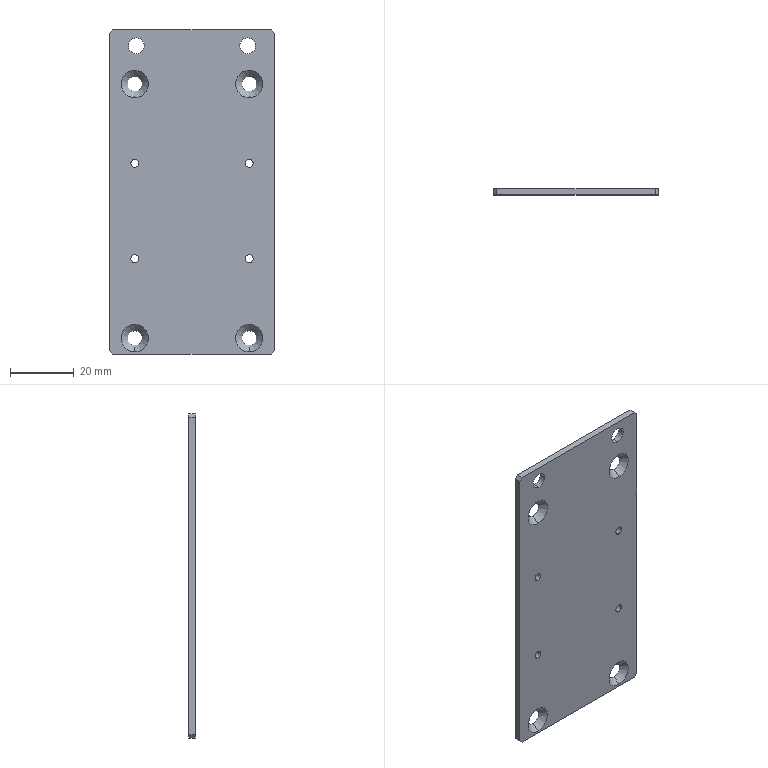Part | STEP file | Push button box mounting base plate | 1 solid | 30 faces | box 52 x 2 x 102 mm | volume 10204 mm3 | cylinder 12 | plane 10 | cone 8 | commonest cylinder face diameters 2.5 x8 5 x4